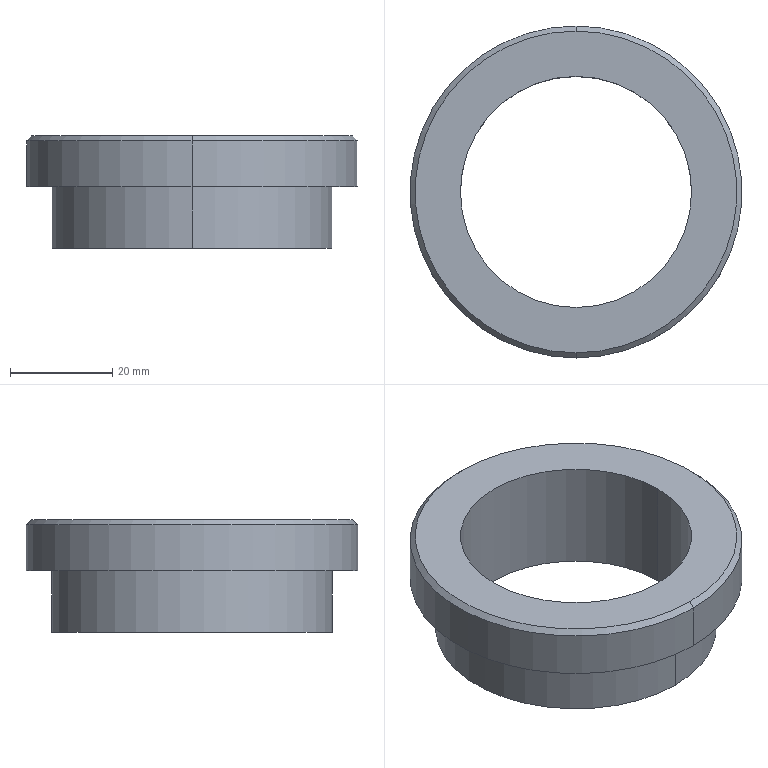Part | SolidWorks | features Chamfer 1, HoleWzd 1, Revolution 1 | 1 solid | 11 faces | box 65 x 65 x 22 mm | volume 26213 mm3 | cylinder 6 | plane 3 | cone 2 | commonest cylinder face diameters 45.25 x2 55 x2 65 x2
STEP:
#1=CARTESIAN_POINT('',(0.,-31.5,22.));
#2=VERTEX_POINT('',#1);
#3=CARTESIAN_POINT('',(0.,31.5,22.));
#4=VERTEX_POINT('',#3);
#5=CARTESIAN_POINT('',(0.,0.,22.));
#6=DIRECTION('',(0.,0.,1.));
#7=DIRECTION('',(0.,1.,0.));
#8=AXIS2_PLACEMENT_3D('',#5,#6,#7);
#9=CIRCLE('',#8,31.5);
#10=EDGE_CURVE('',#2,#4,#9,.T.);
#11=ORIENTED_EDGE('',*,*,#10,.F.);
#12=CARTESIAN_POINT('',(0.,-32.5,21.));
#13=VERTEX_POINT('',#12);
#14=CARTESIAN_POINT('',(0.,-31.5,22.));
#15=DIRECTION('',(0.,-0.7071,-0.7071));
#16=VECTOR('',#15,1000.);
#17=LINE('',#14,#16);
#18=EDGE_CURVE('',#2,#13,#17,.T.);
#19=ORIENTED_EDGE('',*,*,#18,.T.);
#20=CARTESIAN_POINT('',(0.,32.5,21.));
#21=VERTEX_POINT('',#20);
#22=CARTESIAN_POINT('',(0.,0.,21.));
#23=DIRECTION('',(0.,0.,-1.));
#24=DIRECTION('',(0.,1.,0.));
#25=AXIS2_PLACEMENT_3D('',#22,#23,#24);
#26=CIRCLE('',#25,32.5);
#27=EDGE_CURVE('',#21,#13,#26,.T.);
#28=ORIENTED_EDGE('',*,*,#27,.F.);
#29=CARTESIAN_POINT('',(0.,31.5,22.));
#30=DIRECTION('',(0.,0.7071,-0.7071));
#31=VECTOR('',#30,1000.);
#32=LINE('',#29,#31);
#33=EDGE_CURVE('',#4,#21,#32,.T.);
#34=ORIENTED_EDGE('',*,*,#33,.F.);
#35=EDGE_LOOP('',(#11,#19,#28,#34));
#36=FACE_OUTER_BOUND('',#35,.T.);
#37=CARTESIAN_POINT('',(0.,0.,22.));
#38=DIRECTION('',(0.,0.,-1.));
#39=DIRECTION('',(0.,1.,0.));
#40=AXIS2_PLACEMENT_3D('',#37,#38,#39);
#41=CONICAL_SURFACE('',#40,31.5,0.7854);
#42=ADVANCED_FACE('',(#36),#41,.T.);
#43=CARTESIAN_POINT('',(-22.625,0.,0.));
#44=VERTEX_POINT('',#43);
#45=CARTESIAN_POINT('',(22.625,0.,0.));
#46=VERTEX_POINT('',#45);
#47=CARTESIAN_POINT('',(0.,0.,0.));
#48=DIRECTION('',(0.,0.,1.));
#49=DIRECTION('',(1.,0.,0.));
#50=AXIS2_PLACEMENT_3D('',#47,#48,#49);
#51=CIRCLE('',#50,22.625);
#52=EDGE_CURVE('',#44,#46,#51,.T.);
#53=ORIENTED_EDGE('',*,*,#52,.F.);
#54=CARTESIAN_POINT('',(-22.625,0.,22.));
#55=VERTEX_POINT('',#54);
#56=CARTESIAN_POINT('',(-22.625,0.,22.));
#57=DIRECTION('',(0.,0.,1.));
#58=VECTOR('',#57,1000.);
#59=LINE('',#56,#58);
#60=EDGE_CURVE('',#44,#55,#59,.T.);
#61=ORIENTED_EDGE('',*,*,#60,.T.);
#62=CARTESIAN_POINT('',(22.625,0.,22.));
#63=VERTEX_POINT('',#62);
#64=CARTESIAN_POINT('',(0.,0.,22.));
#65=DIRECTION('',(0.,0.,1.));
#66=DIRECTION('',(1.,0.,0.));
#67=AXIS2_PLACEMENT_3D('',#64,#65,#66);
#68=CIRCLE('',#67,22.625);
#69=EDGE_CURVE('',#55,#63,#68,.T.);
#70=ORIENTED_EDGE('',*,*,#69,.T.);
#71=CARTESIAN_POINT('',(22.625,0.,22.));
#72=DIRECTION('',(0.,0.,1.));
#73=VECTOR('',#72,1000.);
#74=LINE('',#71,#73);
#75=EDGE_CURVE('',#46,#63,#74,.T.);
#76=ORIENTED_EDGE('',*,*,#75,.F.);
#77=EDGE_LOOP('',(#53,#61,#70,#76));
#78=FACE_OUTER_BOUND('',#77,.T.);
#79=CARTESIAN_POINT('',(0.,0.,22.));
#80=DIRECTION('',(0.,0.,1.));
#81=DIRECTION('',(1.,0.,0.));
#82=AXIS2_PLACEMENT_3D('',#79,#80,#81);
#83=CYLINDRICAL_SURFACE('',#82,22.625);
#84=ADVANCED_FACE('',(#78),#83,.F.);
#85=CARTESIAN_POINT('',(0.,-32.5,12.));
#86=VERTEX_POINT('',#85);
#87=CARTESIAN_POINT('',(0.,32.5,12.));
#88=VERTEX_POINT('',#87);
#89=CARTESIAN_POINT('',(0.,0.,12.));
#90=DIRECTION('',(0.,0.,1.));
#91=DIRECTION('',(0.,-1.,0.));
#92=AXIS2_PLACEMENT_3D('',#89,#90,#91);
#93=CIRCLE('',#92,32.5);
#94=EDGE_CURVE('',#86,#88,#93,.T.);
#95=ORIENTED_EDGE('',*,*,#94,.T.);
#96=CARTESIAN_POINT('',(0.,32.5,22.));
#97=DIRECTION('',(0.,0.,1.));
#98=VECTOR('',#97,1000.);
#99=LINE('',#96,#98);
#100=EDGE_CURVE('',#88,#21,#99,.T.);
#101=ORIENTED_EDGE('',*,*,#100,.T.);
#102=ORIENTED_EDGE('',*,*,#27,.T.);
#103=CARTESIAN_POINT('',(0.,-32.5,22.));
#104=DIRECTION('',(0.,0.,1.));
#105=VECTOR('',#104,1000.);
#106=LINE('',#103,#105);
#107=EDGE_CURVE('',#86,#13,#106,.T.);
#108=ORIENTED_EDGE('',*,*,#107,.F.);
#109=EDGE_LOOP('',(#95,#101,#102,#108));
#110=FACE_OUTER_BOUND('',#109,.T.);
#111=CARTESIAN_POINT('',(0.,0.,22.));
#112=DIRECTION('',(0.,0.,1.));
#113=DIRECTION('',(0.,-1.,0.));
#114=AXIS2_PLACEMENT_3D('',#111,#112,#113);
#115=CYLINDRICAL_SURFACE('',#114,32.5);
#116=ADVANCED_FACE('',(#110),#115,.T.);
#117=CARTESIAN_POINT('',(0.,-27.5,0.));
#118=VERTEX_POINT('',#117);
#119=CARTESIAN_POINT('',(0.,27.5,0.));
#120=VERTEX_POINT('',#119);
#121=CARTESIAN_POINT('',(0.,0.,0.));
#122=DIRECTION('',(0.,0.,1.));
#123=DIRECTION('',(0.,-1.,0.));
#124=AXIS2_PLACEMENT_3D('',#121,#122,#123);
#125=CIRCLE('',#124,27.5);
#126=EDGE_CURVE('',#118,#120,#125,.T.);
#127=ORIENTED_EDGE('',*,*,#126,.T.);
#128=CARTESIAN_POINT('',(0.,27.5,12.));
#129=VERTEX_POINT('',#128);
#130=CARTESIAN_POINT('',(0.,27.5,22.));
#131=DIRECTION('',(0.,0.,1.));
#132=VECTOR('',#131,1000.);
#133=LINE('',#130,#132);
#134=EDGE_CURVE('',#120,#129,#133,.T.);
#135=ORIENTED_EDGE('',*,*,#134,.T.);
#136=CARTESIAN_POINT('',(0.,-27.5,12.));
#137=VERTEX_POINT('',#136);
#138=CARTESIAN_POINT('',(0.,0.,12.));
#139=DIRECTION('',(0.,0.,1.));
#140=DIRECTION('',(0.,-1.,0.));
#141=AXIS2_PLACEMENT_3D('',#138,#139,#140);
#142=CIRCLE('',#141,27.5);
#143=EDGE_CURVE('',#137,#129,#142,.T.);
#144=ORIENTED_EDGE('',*,*,#143,.F.);
#145=CARTESIAN_POINT('',(0.,-27.5,22.));
#146=DIRECTION('',(0.,0.,1.));
#147=VECTOR('',#146,1000.);
#148=LINE('',#145,#147);
#149=EDGE_CURVE('',#118,#137,#148,.T.);
#150=ORIENTED_EDGE('',*,*,#149,.F.);
#151=EDGE_LOOP('',(#127,#135,#144,#150));
#152=FACE_OUTER_BOUND('',#151,.T.);
#153=CARTESIAN_POINT('',(0.,0.,22.));
#154=DIRECTION('',(0.,0.,1.));
#155=DIRECTION('',(0.,-1.,0.));
#156=AXIS2_PLACEMENT_3D('',#153,#154,#155);
#157=CYLINDRICAL_SURFACE('',#156,27.5);
#158=ADVANCED_FACE('',(#152),#157,.T.);
#159=CARTESIAN_POINT('',(0.,0.,0.));
#160=DIRECTION('',(0.,0.,1.));
#161=DIRECTION('',(1.,0.,0.));
#162=AXIS2_PLACEMENT_3D('',#159,#160,#161);
#163=CIRCLE('',#162,22.625);
#164=EDGE_CURVE('',#46,#44,#163,.T.);
#165=ORIENTED_EDGE('',*,*,#164,.T.);
#166=ORIENTED_EDGE('',*,*,#52,.T.);
#167=EDGE_LOOP('',(#165,#166));
#168=FACE_BOUND('',#167,.T.);
#169=ORIENTED_EDGE('',*,*,#126,.F.);
#170=CARTESIAN_POINT('',(0.,0.,0.));
#171=DIRECTION('',(0.,0.,1.));
#172=DIRECTION('',(0.,-1.,0.));
#173=AXIS2_PLACEMENT_3D('',#170,#171,#172);
#174=CIRCLE('',#173,27.5);
#175=EDGE_CURVE('',#120,#118,#174,.T.);
#176=ORIENTED_EDGE('',*,*,#175,.F.);
#177=EDGE_LOOP('',(#169,#176));
#178=FACE_OUTER_BOUND('',#177,.T.);
#179=CARTESIAN_POINT('',(0.,0.,0.));
#180=DIRECTION('',(0.,0.,1.));
#181=DIRECTION('',(0.,-1.,0.));
#182=AXIS2_PLACEMENT_3D('',#179,#180,#181);
#183=PLANE('',#182);
#184=ADVANCED_FACE('',(#168,#178),#183,.F.);
#185=ORIENTED_EDGE('',*,*,#134,.F.);
#186=ORIENTED_EDGE('',*,*,#175,.T.);
#187=ORIENTED_EDGE('',*,*,#149,.T.);
#188=CARTESIAN_POINT('',(0.,0.,12.));
#189=DIRECTION('',(0.,0.,1.));
#190=DIRECTION('',(0.,-1.,0.));
#191=AXIS2_PLACEMENT_3D('',#188,#189,#190);
#192=CIRCLE('',#191,27.5);
#193=EDGE_CURVE('',#129,#137,#192,.T.);
#194=ORIENTED_EDGE('',*,*,#193,.F.);
#195=EDGE_LOOP('',(#185,#186,#187,#194));
#196=FACE_OUTER_BOUND('',#195,.T.);
#197=CARTESIAN_POINT('',(0.,0.,22.));
#198=DIRECTION('',(0.,0.,1.));
#199=DIRECTION('',(0.,-1.,0.));
#200=AXIS2_PLACEMENT_3D('',#197,#198,#199);
#201=CYLINDRICAL_SURFACE('',#200,27.5);
#202=ADVANCED_FACE('',(#196),#201,.T.);
#203=ORIENTED_EDGE('',*,*,#94,.F.);
#204=CARTESIAN_POINT('',(0.,0.,12.));
#205=DIRECTION('',(0.,0.,1.));
#206=DIRECTION('',(0.,-1.,0.));
#207=AXIS2_PLACEMENT_3D('',#204,#205,#206);
#208=CIRCLE('',#207,32.5);
#209=EDGE_CURVE('',#88,#86,#208,.T.);
#210=ORIENTED_EDGE('',*,*,#209,.F.);
#211=EDGE_LOOP('',(#203,#210));
#212=FACE_OUTER_BOUND('',#211,.T.);
#213=ORIENTED_EDGE('',*,*,#143,.T.);
#214=ORIENTED_EDGE('',*,*,#193,.T.);
#215=EDGE_LOOP('',(#213,#214));
#216=FACE_BOUND('',#215,.T.);
#217=CARTESIAN_POINT('',(0.,27.5,12.));
#218=DIRECTION('',(0.,0.,1.));
#219=DIRECTION('',(0.,-1.,0.));
#220=AXIS2_PLACEMENT_3D('',#217,#218,#219);
#221=PLANE('',#220);
#222=ADVANCED_FACE('',(#212,#216),#221,.F.);
#223=ORIENTED_EDGE('',*,*,#100,.F.);
#224=ORIENTED_EDGE('',*,*,#209,.T.);
#225=ORIENTED_EDGE('',*,*,#107,.T.);
#226=CARTESIAN_POINT('',(0.,0.,21.));
#227=DIRECTION('',(0.,0.,-1.));
#228=DIRECTION('',(0.,1.,0.));
#229=AXIS2_PLACEMENT_3D('',#226,#227,#228);
#230=CIRCLE('',#229,32.5);
#231=EDGE_CURVE('',#13,#21,#230,.T.);
#232=ORIENTED_EDGE('',*,*,#231,.T.);
#233=EDGE_LOOP('',(#223,#224,#225,#232));
#234=FACE_OUTER_BOUND('',#233,.T.);
#235=CARTESIAN_POINT('',(0.,0.,22.));
#236=DIRECTION('',(0.,0.,1.));
#237=DIRECTION('',(0.,-1.,0.));
#238=AXIS2_PLACEMENT_3D('',#235,#236,#237);
#239=CYLINDRICAL_SURFACE('',#238,32.5);
#240=ADVANCED_FACE('',(#234),#239,.T.);
#241=CARTESIAN_POINT('',(0.,0.,22.));
#242=DIRECTION('',(0.,0.,1.));
#243=DIRECTION('',(0.,1.,0.));
#244=AXIS2_PLACEMENT_3D('',#241,#242,#243);
#245=CIRCLE('',#244,31.5);
#246=EDGE_CURVE('',#4,#2,#245,.T.);
#247=ORIENTED_EDGE('',*,*,#246,.T.);
#248=ORIENTED_EDGE('',*,*,#10,.T.);
#249=EDGE_LOOP('',(#247,#248));
#250=FACE_OUTER_BOUND('',#249,.T.);
#251=CARTESIAN_POINT('',(0.,0.,22.));
#252=DIRECTION('',(0.,0.,1.));
#253=DIRECTION('',(1.,0.,0.));
#254=AXIS2_PLACEMENT_3D('',#251,#252,#253);
#255=CIRCLE('',#254,22.625);
#256=EDGE_CURVE('',#63,#55,#255,.T.);
#257=ORIENTED_EDGE('',*,*,#256,.F.);
#258=ORIENTED_EDGE('',*,*,#69,.F.);
#259=EDGE_LOOP('',(#257,#258));
#260=FACE_BOUND('',#259,.T.);
#261=CARTESIAN_POINT('',(0.,32.5,22.));
#262=DIRECTION('',(0.,0.,-1.));
#263=DIRECTION('',(0.,1.,0.));
#264=AXIS2_PLACEMENT_3D('',#261,#262,#263);
#265=PLANE('',#264);
#266=ADVANCED_FACE('',(#250,#260),#265,.F.);
#267=ORIENTED_EDGE('',*,*,#60,.F.);
#268=ORIENTED_EDGE('',*,*,#164,.F.);
#269=ORIENTED_EDGE('',*,*,#75,.T.);
#270=ORIENTED_EDGE('',*,*,#256,.T.);
#271=EDGE_LOOP('',(#267,#268,#269,#270));
#272=FACE_OUTER_BOUND('',#271,.T.);
#273=CARTESIAN_POINT('',(0.,0.,22.));
#274=DIRECTION('',(0.,0.,1.));
#275=DIRECTION('',(1.,0.,0.));
#276=AXIS2_PLACEMENT_3D('',#273,#274,#275);
#277=CYLINDRICAL_SURFACE('',#276,22.625);
#278=ADVANCED_FACE('',(#272),#277,.F.);
#279=ORIENTED_EDGE('',*,*,#18,.F.);
#280=ORIENTED_EDGE('',*,*,#246,.F.);
#281=ORIENTED_EDGE('',*,*,#33,.T.);
#282=ORIENTED_EDGE('',*,*,#231,.F.);
#283=EDGE_LOOP('',(#279,#280,#281,#282));
#284=FACE_OUTER_BOUND('',#283,.T.);
#285=CARTESIAN_POINT('',(0.,0.,22.));
#286=DIRECTION('',(0.,0.,-1.));
#287=DIRECTION('',(0.,1.,0.));
#288=AXIS2_PLACEMENT_3D('',#285,#286,#287);
#289=CONICAL_SURFACE('',#288,31.5,0.7854);
#290=ADVANCED_FACE('',(#284),#289,.T.);
#291=CLOSED_SHELL('',(#42,#84,#116,#158,#184,#202,#222,#240,#266,#278,#290));
#292=MANIFOLD_SOLID_BREP('',#291);
#293=CARTESIAN_POINT('',(0.,0.,0.));
#294=DIRECTION('',(0.,0.,1.));
#295=DIRECTION('',(1.,0.,0.));
#296=AXIS2_PLACEMENT_3D('',#293,#294,#295);
#297=(LENGTH_UNIT()NAMED_UNIT(*)SI_UNIT(.MILLI.,.METRE.));
#298=UNCERTAINTY_MEASURE_WITH_UNIT(LENGTH_MEASURE(0.00001),#297,'','');
#299=(NAMED_UNIT(*)PLANE_ANGLE_UNIT()SI_UNIT($,.RADIAN.));
#300=(NAMED_UNIT(*)SI_UNIT($,.STERADIAN.)SOLID_ANGLE_UNIT());
#301=(GEOMETRIC_REPRESENTATION_CONTEXT(3)GLOBAL_UNCERTAINTY_ASSIGNED_CONTEXT((#298))GLOBAL_UNIT_ASSIGNED_CONTEXT((#297,#299,#300))REPRESENTATION_CONTEXT('',''));
#302=ADVANCED_BREP_SHAPE_REPRESENTATION('',(#292,#296),#301);